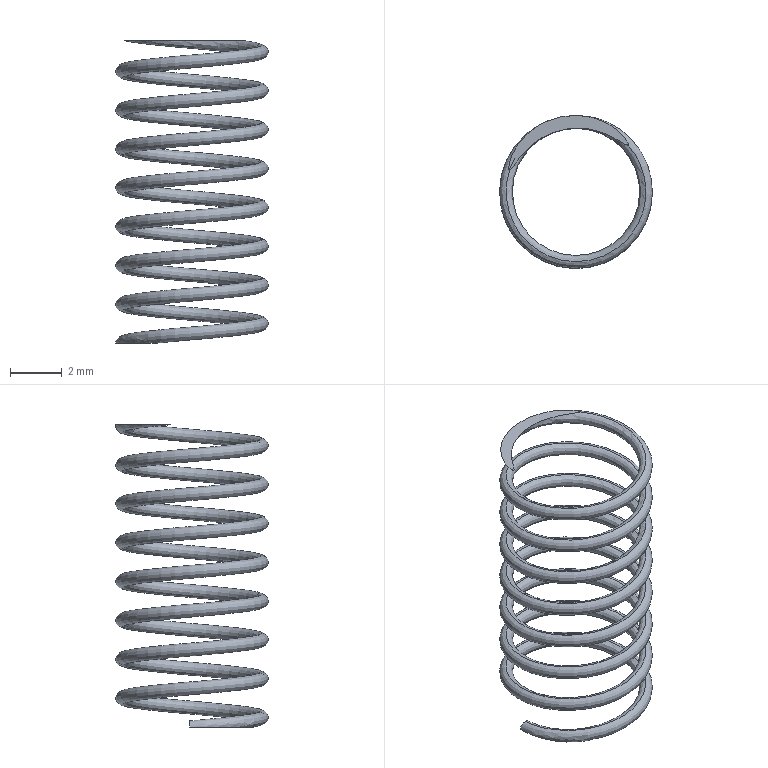Part | SolidWorks | features BaseBody 1 | 1 solid | 5 faces | box 5.9 x 5.9 x 11.683 mm | volume 27.738 mm3 | plane 3 | spline 2